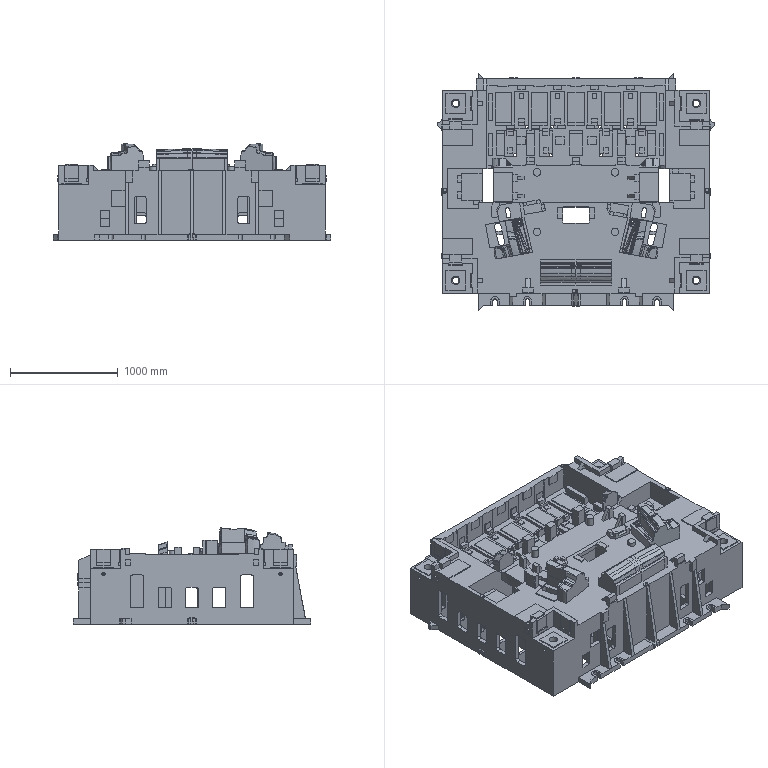Part | NX | features solid 2 | 1 solid | 2977 faces | box 2570 x 2200 x 891.336 mm | volume 861715869 mm3 | plane 2078 | cylinder 537 | spline 359 | cone 3 | commonest cylinder face diameters 40 x464 30 x18 80 x12 60 x10 10 x9 4 x4